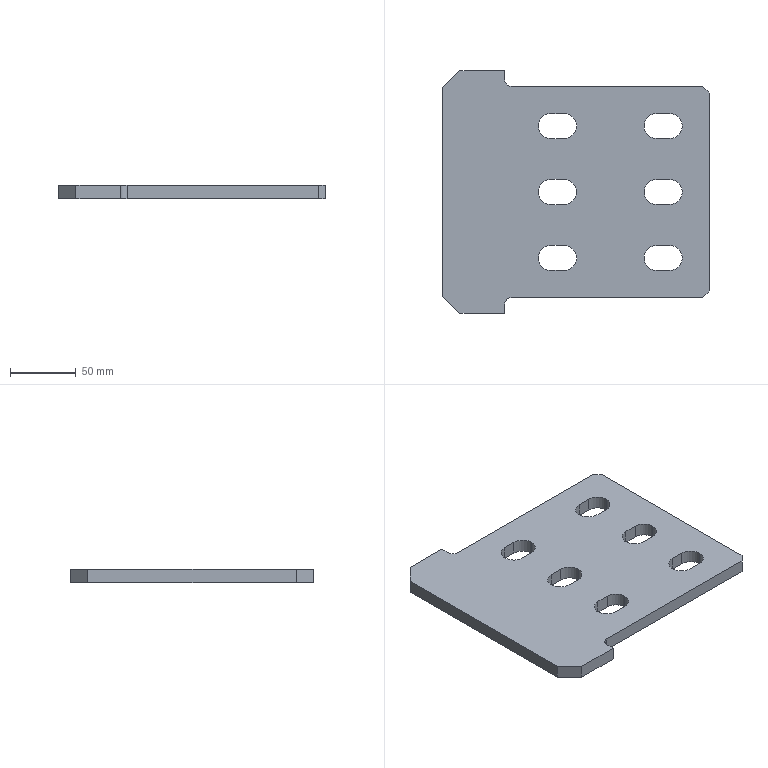Part | STEP file | 筋Plate-200×100-200 | 1 solid | 46 faces | box 202 x 184 x 10 mm | volume 304236 mm3 | plane 26 | cylinder 20 | commonest cylinder face diameters 19 x18 10 x2